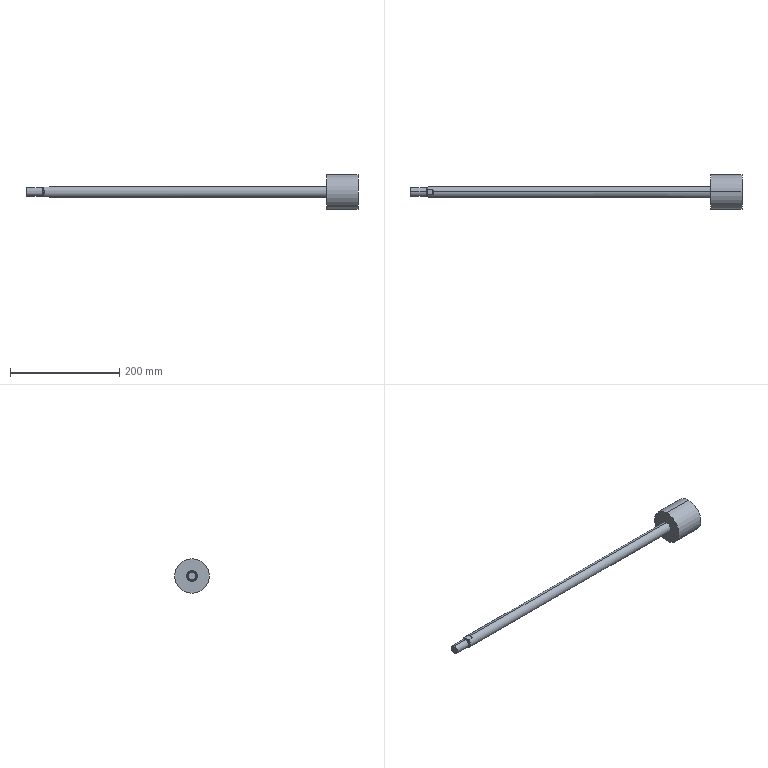Part | SolidWorks | features BaseBody 1 | 1 solid | 21 faces | box 608 x 63 x 63 mm | volume 346803 mm3 | plane 9 | cylinder 8 | cone 4 | commonest cylinder face diameters 14 x2 16 x2 20 x2 63 x2
STEP:
#1=CARTESIAN_POINT('',(482.,0.,10.));
#2=VERTEX_POINT('',#1);
#3=CARTESIAN_POINT('',(482.,0.,-10.));
#4=VERTEX_POINT('',#3);
#5=CARTESIAN_POINT('',(482.,0.,0.));
#6=DIRECTION('',(-1.,0.,0.));
#7=DIRECTION('',(0.,0.,1.));
#8=AXIS2_PLACEMENT_3D('',#5,#6,#7);
#9=CIRCLE('',#8,10.);
#10=EDGE_CURVE('',#2,#4,#9,.T.);
#11=ORIENTED_EDGE('',*,*,#10,.T.);
#12=CARTESIAN_POINT('',(-25.5,0.,-10.));
#13=VERTEX_POINT('',#12);
#14=CARTESIAN_POINT('',(539.,0.,-10.));
#15=DIRECTION('',(-1.,0.,0.));
#16=VECTOR('',#15,1000.);
#17=LINE('',#14,#16);
#18=EDGE_CURVE('',#4,#13,#17,.T.);
#19=ORIENTED_EDGE('',*,*,#18,.T.);
#20=CARTESIAN_POINT('',(-27.,5.268,-8.5));
#21=VERTEX_POINT('',#20);
#22=CARTESIAN_POINT('',(-25.5,0.,-10.));
#23=CARTESIAN_POINT('',(-25.5,1.873,-10.));
#24=CARTESIAN_POINT('',(-26.013,3.675,-9.487));
#25=CARTESIAN_POINT('',(-27.,5.268,-8.5));
#26=(BOUNDED_CURVE()B_SPLINE_CURVE(3,(#22,#23,#24,#25),.UNSPECIFIED.,.F.,.F.)B_SPLINE_CURVE_WITH_KNOTS((4,4),(3.142,3.696),.UNSPECIFIED.)CURVE()GEOMETRIC_REPRESENTATION_ITEM()RATIONAL_B_SPLINE_CURVE((1.,0.9745,0.9745,1.))REPRESENTATION_ITEM(''));
#27=EDGE_CURVE('',#13,#21,#26,.T.);
#28=ORIENTED_EDGE('',*,*,#27,.T.);
#29=CARTESIAN_POINT('',(-36.,5.268,-8.5));
#30=VERTEX_POINT('',#29);
#31=CARTESIAN_POINT('',(539.,5.268,-8.5));
#32=DIRECTION('',(-1.,0.,0.));
#33=VECTOR('',#32,1000.);
#34=LINE('',#31,#33);
#35=EDGE_CURVE('',#21,#30,#34,.T.);
#36=ORIENTED_EDGE('',*,*,#35,.T.);
#37=CARTESIAN_POINT('',(-36.,5.268,8.5));
#38=VERTEX_POINT('',#37);
#39=CARTESIAN_POINT('',(-36.,0.,0.));
#40=DIRECTION('',(1.,0.,0.));
#41=DIRECTION('',(0.,0.,1.));
#42=AXIS2_PLACEMENT_3D('',#39,#40,#41);
#43=CIRCLE('',#42,10.);
#44=EDGE_CURVE('',#30,#38,#43,.T.);
#45=ORIENTED_EDGE('',*,*,#44,.T.);
#46=CARTESIAN_POINT('',(-27.,5.268,8.5));
#47=VERTEX_POINT('',#46);
#48=CARTESIAN_POINT('',(539.,5.268,8.5));
#49=DIRECTION('',(1.,0.,0.));
#50=VECTOR('',#49,1000.);
#51=LINE('',#48,#50);
#52=EDGE_CURVE('',#38,#47,#51,.T.);
#53=ORIENTED_EDGE('',*,*,#52,.T.);
#54=CARTESIAN_POINT('',(-25.5,0.,10.));
#55=VERTEX_POINT('',#54);
#56=CARTESIAN_POINT('',(-27.,5.268,8.5));
#57=CARTESIAN_POINT('',(-26.013,3.675,9.487));
#58=CARTESIAN_POINT('',(-25.5,1.873,10.));
#59=CARTESIAN_POINT('',(-25.5,0.,10.));
#60=(BOUNDED_CURVE()B_SPLINE_CURVE(3,(#56,#57,#58,#59),.UNSPECIFIED.,.F.,.F.)B_SPLINE_CURVE_WITH_KNOTS((4,4),(2.587,3.142),.UNSPECIFIED.)CURVE()GEOMETRIC_REPRESENTATION_ITEM()RATIONAL_B_SPLINE_CURVE((1.,0.9745,0.9745,1.))REPRESENTATION_ITEM(''));
#61=EDGE_CURVE('',#47,#55,#60,.T.);
#62=ORIENTED_EDGE('',*,*,#61,.T.);
#63=CARTESIAN_POINT('',(539.,0.,10.));
#64=DIRECTION('',(-1.,0.,0.));
#65=VECTOR('',#64,1000.);
#66=LINE('',#63,#65);
#67=EDGE_CURVE('',#2,#55,#66,.T.);
#68=ORIENTED_EDGE('',*,*,#67,.F.);
#69=EDGE_LOOP('',(#11,#19,#28,#36,#45,#53,#62,#68));
#70=FACE_OUTER_BOUND('',#69,.T.);
#71=CARTESIAN_POINT('',(539.,0.,0.));
#72=DIRECTION('',(-1.,0.,0.));
#73=DIRECTION('',(0.,0.,1.));
#74=AXIS2_PLACEMENT_3D('',#71,#72,#73);
#75=CYLINDRICAL_SURFACE('',#74,10.);
#76=ADVANCED_FACE('',(#70),#75,.T.);
#77=CARTESIAN_POINT('',(539.,0.,31.5));
#78=VERTEX_POINT('',#77);
#79=CARTESIAN_POINT('',(539.,0.,-31.5));
#80=VERTEX_POINT('',#79);
#81=CARTESIAN_POINT('',(539.,0.,0.));
#82=DIRECTION('',(-1.,0.,0.));
#83=DIRECTION('',(0.,0.,1.));
#84=AXIS2_PLACEMENT_3D('',#81,#82,#83);
#85=CIRCLE('',#84,31.5);
#86=EDGE_CURVE('',#78,#80,#85,.T.);
#87=ORIENTED_EDGE('',*,*,#86,.T.);
#88=CARTESIAN_POINT('',(482.,0.,-31.5));
#89=VERTEX_POINT('',#88);
#90=CARTESIAN_POINT('',(539.,0.,-31.5));
#91=DIRECTION('',(-1.,0.,0.));
#92=VECTOR('',#91,1000.);
#93=LINE('',#90,#92);
#94=EDGE_CURVE('',#80,#89,#93,.T.);
#95=ORIENTED_EDGE('',*,*,#94,.T.);
#96=CARTESIAN_POINT('',(482.,0.,31.5));
#97=VERTEX_POINT('',#96);
#98=CARTESIAN_POINT('',(482.,0.,0.));
#99=DIRECTION('',(1.,0.,0.));
#100=DIRECTION('',(0.,0.,1.));
#101=AXIS2_PLACEMENT_3D('',#98,#99,#100);
#102=CIRCLE('',#101,31.5);
#103=EDGE_CURVE('',#89,#97,#102,.T.);
#104=ORIENTED_EDGE('',*,*,#103,.T.);
#105=CARTESIAN_POINT('',(539.,0.,31.5));
#106=DIRECTION('',(-1.,0.,0.));
#107=VECTOR('',#106,1000.);
#108=LINE('',#105,#107);
#109=EDGE_CURVE('',#78,#97,#108,.T.);
#110=ORIENTED_EDGE('',*,*,#109,.F.);
#111=EDGE_LOOP('',(#87,#95,#104,#110));
#112=FACE_OUTER_BOUND('',#111,.T.);
#113=CARTESIAN_POINT('',(539.,0.,0.));
#114=DIRECTION('',(-1.,0.,0.));
#115=DIRECTION('',(0.,0.,1.));
#116=AXIS2_PLACEMENT_3D('',#113,#114,#115);
#117=CYLINDRICAL_SURFACE('',#116,31.5);
#118=ADVANCED_FACE('',(#112),#117,.T.);
#119=CARTESIAN_POINT('',(-37.,0.,7.));
#120=VERTEX_POINT('',#119);
#121=CARTESIAN_POINT('',(-37.,0.,-7.));
#122=VERTEX_POINT('',#121);
#123=CARTESIAN_POINT('',(-37.,0.,0.));
#124=DIRECTION('',(-1.,0.,0.));
#125=DIRECTION('',(0.,0.,1.));
#126=AXIS2_PLACEMENT_3D('',#123,#124,#125);
#127=CIRCLE('',#126,7.);
#128=EDGE_CURVE('',#120,#122,#127,.T.);
#129=ORIENTED_EDGE('',*,*,#128,.T.);
#130=CARTESIAN_POINT('',(-39.,0.,-7.));
#131=VERTEX_POINT('',#130);
#132=CARTESIAN_POINT('',(539.,0.,-7.));
#133=DIRECTION('',(-1.,0.,0.));
#134=VECTOR('',#133,1000.);
#135=LINE('',#132,#134);
#136=EDGE_CURVE('',#122,#131,#135,.T.);
#137=ORIENTED_EDGE('',*,*,#136,.T.);
#138=CARTESIAN_POINT('',(-39.,0.,7.));
#139=VERTEX_POINT('',#138);
#140=CARTESIAN_POINT('',(-39.,0.,0.));
#141=DIRECTION('',(1.,0.,0.));
#142=DIRECTION('',(0.,0.,1.));
#143=AXIS2_PLACEMENT_3D('',#140,#141,#142);
#144=CIRCLE('',#143,7.);
#145=EDGE_CURVE('',#131,#139,#144,.T.);
#146=ORIENTED_EDGE('',*,*,#145,.T.);
#147=CARTESIAN_POINT('',(539.,0.,7.));
#148=DIRECTION('',(-1.,0.,0.));
#149=VECTOR('',#148,1000.);
#150=LINE('',#147,#149);
#151=EDGE_CURVE('',#120,#139,#150,.T.);
#152=ORIENTED_EDGE('',*,*,#151,.F.);
#153=EDGE_LOOP('',(#129,#137,#146,#152));
#154=FACE_OUTER_BOUND('',#153,.T.);
#155=CARTESIAN_POINT('',(539.,0.,0.));
#156=DIRECTION('',(-1.,0.,0.));
#157=DIRECTION('',(0.,0.,1.));
#158=AXIS2_PLACEMENT_3D('',#155,#156,#157);
#159=CYLINDRICAL_SURFACE('',#158,7.);
#160=ADVANCED_FACE('',(#154),#159,.T.);
#161=CARTESIAN_POINT('',(-39.,0.,8.));
#162=VERTEX_POINT('',#161);
#163=CARTESIAN_POINT('',(-39.,0.,-8.));
#164=VERTEX_POINT('',#163);
#165=CARTESIAN_POINT('',(-39.,0.,0.));
#166=DIRECTION('',(-1.,0.,0.));
#167=DIRECTION('',(0.,0.,1.));
#168=AXIS2_PLACEMENT_3D('',#165,#166,#167);
#169=CIRCLE('',#168,8.);
#170=EDGE_CURVE('',#162,#164,#169,.T.);
#171=ORIENTED_EDGE('',*,*,#170,.T.);
#172=CARTESIAN_POINT('',(-68.08,0.,-8.));
#173=VERTEX_POINT('',#172);
#174=CARTESIAN_POINT('',(539.,0.,-8.));
#175=DIRECTION('',(-1.,0.,0.));
#176=VECTOR('',#175,1000.);
#177=LINE('',#174,#176);
#178=EDGE_CURVE('',#164,#173,#177,.T.);
#179=ORIENTED_EDGE('',*,*,#178,.T.);
#180=CARTESIAN_POINT('',(-68.08,0.,8.));
#181=VERTEX_POINT('',#180);
#182=CARTESIAN_POINT('',(-68.08,0.,0.));
#183=DIRECTION('',(1.,0.,0.));
#184=DIRECTION('',(0.,0.,1.));
#185=AXIS2_PLACEMENT_3D('',#182,#183,#184);
#186=CIRCLE('',#185,8.);
#187=EDGE_CURVE('',#173,#181,#186,.T.);
#188=ORIENTED_EDGE('',*,*,#187,.T.);
#189=CARTESIAN_POINT('',(539.,0.,8.));
#190=DIRECTION('',(-1.,0.,0.));
#191=VECTOR('',#190,1000.);
#192=LINE('',#189,#191);
#193=EDGE_CURVE('',#162,#181,#192,.T.);
#194=ORIENTED_EDGE('',*,*,#193,.F.);
#195=EDGE_LOOP('',(#171,#179,#188,#194));
#196=FACE_OUTER_BOUND('',#195,.T.);
#197=CARTESIAN_POINT('',(539.,0.,0.));
#198=DIRECTION('',(-1.,0.,0.));
#199=DIRECTION('',(0.,0.,1.));
#200=AXIS2_PLACEMENT_3D('',#197,#198,#199);
#201=CYLINDRICAL_SURFACE('',#200,8.);
#202=ADVANCED_FACE('',(#196),#201,.T.);
#203=CARTESIAN_POINT('',(-69.,0.,-7.08));
#204=VERTEX_POINT('',#203);
#205=CARTESIAN_POINT('',(-69.,0.,7.08));
#206=VERTEX_POINT('',#205);
#207=CARTESIAN_POINT('',(-69.,0.,0.));
#208=DIRECTION('',(1.,0.,0.));
#209=DIRECTION('',(0.,0.,-1.));
#210=AXIS2_PLACEMENT_3D('',#207,#208,#209);
#211=CIRCLE('',#210,7.08);
#212=EDGE_CURVE('',#204,#206,#211,.T.);
#213=ORIENTED_EDGE('',*,*,#212,.T.);
#214=CARTESIAN_POINT('',(-68.08,0.,8.));
#215=DIRECTION('',(0.7071,0.,0.7071));
#216=VECTOR('',#215,1000.);
#217=LINE('',#214,#216);
#218=EDGE_CURVE('',#206,#181,#217,.T.);
#219=ORIENTED_EDGE('',*,*,#218,.T.);
#220=ORIENTED_EDGE('',*,*,#187,.F.);
#221=CARTESIAN_POINT('',(-68.08,0.,-8.));
#222=DIRECTION('',(0.7071,0.,-0.7071));
#223=VECTOR('',#222,1000.);
#224=LINE('',#221,#223);
#225=EDGE_CURVE('',#204,#173,#224,.T.);
#226=ORIENTED_EDGE('',*,*,#225,.F.);
#227=EDGE_LOOP('',(#213,#219,#220,#226));
#228=FACE_OUTER_BOUND('',#227,.T.);
#229=CARTESIAN_POINT('',(-68.08,0.,0.));
#230=DIRECTION('',(1.,0.,0.));
#231=DIRECTION('',(0.,0.,-1.));
#232=AXIS2_PLACEMENT_3D('',#229,#230,#231);
#233=CONICAL_SURFACE('',#232,8.,0.7854);
#234=ADVANCED_FACE('',(#228),#233,.T.);
#235=ORIENTED_EDGE('',*,*,#18,.F.);
#236=CARTESIAN_POINT('',(482.,0.,0.));
#237=DIRECTION('',(-1.,0.,0.));
#238=DIRECTION('',(0.,0.,1.));
#239=AXIS2_PLACEMENT_3D('',#236,#237,#238);
#240=CIRCLE('',#239,10.);
#241=EDGE_CURVE('',#4,#2,#240,.T.);
#242=ORIENTED_EDGE('',*,*,#241,.T.);
#243=ORIENTED_EDGE('',*,*,#67,.T.);
#244=CARTESIAN_POINT('',(-27.,-5.268,8.5));
#245=VERTEX_POINT('',#244);
#246=CARTESIAN_POINT('',(-25.5,0.,10.));
#247=CARTESIAN_POINT('',(-25.5,-1.873,10.));
#248=CARTESIAN_POINT('',(-26.013,-3.675,9.487));
#249=CARTESIAN_POINT('',(-27.,-5.268,8.5));
#250=(BOUNDED_CURVE()B_SPLINE_CURVE(3,(#246,#247,#248,#249),.UNSPECIFIED.,.F.,.F.)B_SPLINE_CURVE_WITH_KNOTS((4,4),(3.142,3.696),.UNSPECIFIED.)CURVE()GEOMETRIC_REPRESENTATION_ITEM()RATIONAL_B_SPLINE_CURVE((1.,0.9745,0.9745,1.))REPRESENTATION_ITEM(''));
#251=EDGE_CURVE('',#55,#245,#250,.T.);
#252=ORIENTED_EDGE('',*,*,#251,.T.);
#253=CARTESIAN_POINT('',(-36.,-5.268,8.5));
#254=VERTEX_POINT('',#253);
#255=CARTESIAN_POINT('',(539.,-5.268,8.5));
#256=DIRECTION('',(-1.,0.,0.));
#257=VECTOR('',#256,1000.);
#258=LINE('',#255,#257);
#259=EDGE_CURVE('',#245,#254,#258,.T.);
#260=ORIENTED_EDGE('',*,*,#259,.T.);
#261=CARTESIAN_POINT('',(-36.,-5.268,-8.5));
#262=VERTEX_POINT('',#261);
#263=CARTESIAN_POINT('',(-36.,0.,0.));
#264=DIRECTION('',(1.,0.,0.));
#265=DIRECTION('',(0.,0.,1.));
#266=AXIS2_PLACEMENT_3D('',#263,#264,#265);
#267=CIRCLE('',#266,10.);
#268=EDGE_CURVE('',#254,#262,#267,.T.);
#269=ORIENTED_EDGE('',*,*,#268,.T.);
#270=CARTESIAN_POINT('',(-27.,-5.268,-8.5));
#271=VERTEX_POINT('',#270);
#272=CARTESIAN_POINT('',(539.,-5.268,-8.5));
#273=DIRECTION('',(1.,0.,0.));
#274=VECTOR('',#273,1000.);
#275=LINE('',#272,#274);
#276=EDGE_CURVE('',#262,#271,#275,.T.);
#277=ORIENTED_EDGE('',*,*,#276,.T.);
#278=CARTESIAN_POINT('',(-27.,-5.268,-8.5));
#279=CARTESIAN_POINT('',(-26.013,-3.675,-9.487));
#280=CARTESIAN_POINT('',(-25.5,-1.873,-10.));
#281=CARTESIAN_POINT('',(-25.5,0.,-10.));
#282=(BOUNDED_CURVE()B_SPLINE_CURVE(3,(#278,#279,#280,#281),.UNSPECIFIED.,.F.,.F.)B_SPLINE_CURVE_WITH_KNOTS((4,4),(2.587,3.142),.UNSPECIFIED.)CURVE()GEOMETRIC_REPRESENTATION_ITEM()RATIONAL_B_SPLINE_CURVE((1.,0.9745,0.9745,1.))REPRESENTATION_ITEM(''));
#283=EDGE_CURVE('',#271,#13,#282,.T.);
#284=ORIENTED_EDGE('',*,*,#283,.T.);
#285=EDGE_LOOP('',(#235,#242,#243,#252,#260,#269,#277,#284));
#286=FACE_OUTER_BOUND('',#285,.T.);
#287=CARTESIAN_POINT('',(539.,0.,0.));
#288=DIRECTION('',(-1.,0.,0.));
#289=DIRECTION('',(0.,0.,1.));
#290=AXIS2_PLACEMENT_3D('',#287,#288,#289);
#291=CYLINDRICAL_SURFACE('',#290,10.);
#292=ADVANCED_FACE('',(#286),#291,.T.);
#293=ORIENTED_EDGE('',*,*,#61,.F.);
#294=CARTESIAN_POINT('',(-27.,20.,8.5));
#295=DIRECTION('',(0.,-1.,0.));
#296=VECTOR('',#295,1000.);
#297=LINE('',#294,#296);
#298=EDGE_CURVE('',#47,#245,#297,.T.);
#299=ORIENTED_EDGE('',*,*,#298,.T.);
#300=ORIENTED_EDGE('',*,*,#251,.F.);
#301=EDGE_LOOP('',(#293,#299,#300));
#302=FACE_OUTER_BOUND('',#301,.T.);
#303=CARTESIAN_POINT('',(-11.393,20.,24.107));
#304=DIRECTION('',(-0.7071,0.,0.7071));
#305=DIRECTION('',(0.7071,0.,0.7071));
#306=AXIS2_PLACEMENT_3D('',#303,#304,#305);
#307=PLANE('',#306);
#308=ADVANCED_FACE('',(#302),#307,.T.);
#309=CARTESIAN_POINT('',(-37.,2.958,8.5));
#310=VERTEX_POINT('',#309);
#311=CARTESIAN_POINT('',(-36.,5.268,8.5));
#312=CARTESIAN_POINT('',(-36.392,4.523,8.5));
#313=CARTESIAN_POINT('',(-36.737,3.758,8.5));
#314=CARTESIAN_POINT('',(-37.,2.958,8.5));
#315=B_SPLINE_CURVE_WITH_KNOTS('',3,(#311,#312,#313,#314),.UNSPECIFIED.,.F.,.F.,(4,4),(0.,0.002517),.UNSPECIFIED.);
#316=EDGE_CURVE('',#38,#310,#315,.T.);
#317=ORIENTED_EDGE('',*,*,#316,.T.);
#318=CARTESIAN_POINT('',(-37.,-2.958,8.5));
#319=VERTEX_POINT('',#318);
#320=CARTESIAN_POINT('',(-37.,20.,8.5));
#321=DIRECTION('',(0.,-1.,0.));
#322=VECTOR('',#321,1000.);
#323=LINE('',#320,#322);
#324=EDGE_CURVE('',#310,#319,#323,.T.);
#325=ORIENTED_EDGE('',*,*,#324,.T.);
#326=CARTESIAN_POINT('',(-37.,-2.958,8.5));
#327=CARTESIAN_POINT('',(-36.737,-3.758,8.5));
#328=CARTESIAN_POINT('',(-36.392,-4.523,8.5));
#329=CARTESIAN_POINT('',(-36.,-5.268,8.5));
#330=B_SPLINE_CURVE_WITH_KNOTS('',3,(#326,#327,#328,#329),.UNSPECIFIED.,.F.,.F.,(4,4),(0.,0.002517),.UNSPECIFIED.);
#331=EDGE_CURVE('',#319,#254,#330,.T.);
#332=ORIENTED_EDGE('',*,*,#331,.T.);
#333=ORIENTED_EDGE('',*,*,#259,.F.);
#334=ORIENTED_EDGE('',*,*,#298,.F.);
#335=ORIENTED_EDGE('',*,*,#52,.F.);
#336=EDGE_LOOP('',(#317,#325,#332,#333,#334,#335));
#337=FACE_OUTER_BOUND('',#336,.T.);
#338=CARTESIAN_POINT('',(-27.,20.,8.5));
#339=DIRECTION('',(0.,0.,1.));
#340=DIRECTION('',(1.,0.,0.));
#341=AXIS2_PLACEMENT_3D('',#338,#339,#340);
#342=PLANE('',#341);
#343=ADVANCED_FACE('',(#337),#342,.T.);
#344=ORIENTED_EDGE('',*,*,#316,.F.);
#345=ORIENTED_EDGE('',*,*,#44,.F.);
#346=CARTESIAN_POINT('',(-37.,2.958,-8.5));
#347=VERTEX_POINT('',#346);
#348=CARTESIAN_POINT('',(-36.,5.268,-8.5));
#349=CARTESIAN_POINT('',(-36.392,4.523,-8.5));
#350=CARTESIAN_POINT('',(-36.737,3.758,-8.5));
#351=CARTESIAN_POINT('',(-37.,2.958,-8.5));
#352=B_SPLINE_CURVE_WITH_KNOTS('',3,(#348,#349,#350,#351),.UNSPECIFIED.,.F.,.F.,(4,4),(0.,0.002517),.UNSPECIFIED.);
#353=EDGE_CURVE('',#30,#347,#352,.T.);
#354=ORIENTED_EDGE('',*,*,#353,.T.);
#355=CARTESIAN_POINT('',(-37.,0.,0.));
#356=DIRECTION('',(1.,0.,0.));
#357=DIRECTION('',(0.,0.,-1.));
#358=AXIS2_PLACEMENT_3D('',#355,#356,#357);
#359=CIRCLE('',#358,9.);
#360=EDGE_CURVE('',#347,#310,#359,.T.);
#361=ORIENTED_EDGE('',*,*,#360,.T.);
#362=EDGE_LOOP('',(#344,#345,#354,#361));
#363=FACE_OUTER_BOUND('',#362,.T.);
#364=CARTESIAN_POINT('',(-36.,0.,0.));
#365=DIRECTION('',(1.,0.,0.));
#366=DIRECTION('',(0.,0.,-1.));
#367=AXIS2_PLACEMENT_3D('',#364,#365,#366);
#368=CONICAL_SURFACE('',#367,10.,0.7854);
#369=ADVANCED_FACE('',(#363),#368,.T.);
#370=CARTESIAN_POINT('',(-37.,-2.958,-8.5));
#371=VERTEX_POINT('',#370);
#372=CARTESIAN_POINT('',(-36.,-5.268,-8.5));
#373=CARTESIAN_POINT('',(-36.392,-4.523,-8.5));
#374=CARTESIAN_POINT('',(-36.737,-3.758,-8.5));
#375=CARTESIAN_POINT('',(-37.,-2.958,-8.5));
#376=B_SPLINE_CURVE_WITH_KNOTS('',3,(#372,#373,#374,#375),.UNSPECIFIED.,.F.,.F.,(4,4),(0.,0.002517),.UNSPECIFIED.);
#377=EDGE_CURVE('',#262,#371,#376,.T.);
#378=ORIENTED_EDGE('',*,*,#377,.T.);
#379=CARTESIAN_POINT('',(-37.,20.,-8.5));
#380=DIRECTION('',(0.,1.,0.));
#381=VECTOR('',#380,1000.);
#382=LINE('',#379,#381);
#383=EDGE_CURVE('',#371,#347,#382,.T.);
#384=ORIENTED_EDGE('',*,*,#383,.T.);
#385=ORIENTED_EDGE('',*,*,#353,.F.);
#386=ORIENTED_EDGE('',*,*,#35,.F.);
#387=CARTESIAN_POINT('',(-27.,20.,-8.5));
#388=DIRECTION('',(0.,-1.,0.));
#389=VECTOR('',#388,1000.);
#390=LINE('',#387,#389);
#391=EDGE_CURVE('',#21,#271,#390,.T.);
#392=ORIENTED_EDGE('',*,*,#391,.T.);
#393=ORIENTED_EDGE('',*,*,#276,.F.);
#394=EDGE_LOOP('',(#378,#384,#385,#386,#392,#393));
#395=FACE_OUTER_BOUND('',#394,.T.);
#396=CARTESIAN_POINT('',(-37.,20.,-8.5));
#397=DIRECTION('',(0.,0.,-1.));
#398=DIRECTION('',(-1.,0.,0.));
#399=AXIS2_PLACEMENT_3D('',#396,#397,#398);
#400=PLANE('',#399);
#401=ADVANCED_FACE('',(#395),#400,.T.);
#402=ORIENTED_EDGE('',*,*,#283,.F.);
#403=ORIENTED_EDGE('',*,*,#391,.F.);
#404=ORIENTED_EDGE('',*,*,#27,.F.);
#405=EDGE_LOOP('',(#402,#403,#404));
#406=FACE_OUTER_BOUND('',#405,.T.);
#407=CARTESIAN_POINT('',(-27.,20.,-8.5));
#408=DIRECTION('',(-0.7071,0.,-0.7071));
#409=DIRECTION('',(-0.7071,0.,0.7071));
#410=AXIS2_PLACEMENT_3D('',#407,#408,#409);
#411=PLANE('',#410);
#412=ADVANCED_FACE('',(#406),#411,.T.);
#413=ORIENTED_EDGE('',*,*,#377,.F.);
#414=ORIENTED_EDGE('',*,*,#268,.F.);
#415=ORIENTED_EDGE('',*,*,#331,.F.);
#416=CARTESIAN_POINT('',(-37.,0.,0.));
#417=DIRECTION('',(1.,0.,0.));
#418=DIRECTION('',(0.,0.,-1.));
#419=AXIS2_PLACEMENT_3D('',#416,#417,#418);
#420=CIRCLE('',#419,9.);
#421=EDGE_CURVE('',#319,#371,#420,.T.);
#422=ORIENTED_EDGE('',*,*,#421,.T.);
#423=EDGE_LOOP('',(#413,#414,#415,#422));
#424=FACE_OUTER_BOUND('',#423,.T.);
#425=CARTESIAN_POINT('',(-36.,0.,0.));
#426=DIRECTION('',(1.,0.,0.));
#427=DIRECTION('',(0.,0.,-1.));
#428=AXIS2_PLACEMENT_3D('',#425,#426,#427);
#429=CONICAL_SURFACE('',#428,10.,0.7854);
#430=ADVANCED_FACE('',(#424),#429,.T.);
#431=ORIENTED_EDGE('',*,*,#10,.F.);
#432=ORIENTED_EDGE('',*,*,#241,.F.);
#433=EDGE_LOOP('',(#431,#432));
#434=FACE_BOUND('',#433,.T.);
#435=CARTESIAN_POINT('',(482.,0.,0.));
#436=DIRECTION('',(1.,0.,0.));
#437=DIRECTION('',(0.,0.,1.));
#438=AXIS2_PLACEMENT_3D('',#435,#436,#437);
#439=CIRCLE('',#438,31.5);
#440=EDGE_CURVE('',#97,#89,#439,.T.);
#441=ORIENTED_EDGE('',*,*,#440,.F.);
#442=ORIENTED_EDGE('',*,*,#103,.F.);
#443=EDGE_LOOP('',(#441,#442));
#444=FACE_OUTER_BOUND('',#443,.T.);
#445=CARTESIAN_POINT('',(482.,10.,0.));
#446=DIRECTION('',(1.,0.,0.));
#447=DIRECTION('',(0.,0.,-1.));
#448=AXIS2_PLACEMENT_3D('',#445,#446,#447);
#449=PLANE('',#448);
#450=ADVANCED_FACE('',(#434,#444),#449,.F.);
#451=ORIENTED_EDGE('',*,*,#128,.F.);
#452=CARTESIAN_POINT('',(-37.,0.,0.));
#453=DIRECTION('',(-1.,0.,0.));
#454=DIRECTION('',(0.,0.,1.));
#455=AXIS2_PLACEMENT_3D('',#452,#453,#454);
#456=CIRCLE('',#455,7.);
#457=EDGE_CURVE('',#122,#120,#456,.T.);
#458=ORIENTED_EDGE('',*,*,#457,.F.);
#459=EDGE_LOOP('',(#451,#458));
#460=FACE_BOUND('',#459,.T.);
#461=ORIENTED_EDGE('',*,*,#383,.F.);
#462=ORIENTED_EDGE('',*,*,#421,.F.);
#463=ORIENTED_EDGE('',*,*,#324,.F.);
#464=ORIENTED_EDGE('',*,*,#360,.F.);
#465=EDGE_LOOP('',(#461,#462,#463,#464));
#466=FACE_OUTER_BOUND('',#465,.T.);
#467=CARTESIAN_POINT('',(-37.,7.,0.));
#468=DIRECTION('',(1.,0.,0.));
#469=DIRECTION('',(0.,0.,-1.));
#470=AXIS2_PLACEMENT_3D('',#467,#468,#469);
#471=PLANE('',#470);
#472=ADVANCED_FACE('',(#460,#466),#471,.F.);
#473=ORIENTED_EDGE('',*,*,#94,.F.);
#474=CARTESIAN_POINT('',(539.,0.,0.));
#475=DIRECTION('',(-1.,0.,0.));
#476=DIRECTION('',(0.,0.,1.));
#477=AXIS2_PLACEMENT_3D('',#474,#475,#476);
#478=CIRCLE('',#477,31.5);
#479=EDGE_CURVE('',#80,#78,#478,.T.);
#480=ORIENTED_EDGE('',*,*,#479,.T.);
#481=ORIENTED_EDGE('',*,*,#109,.T.);
#482=ORIENTED_EDGE('',*,*,#440,.T.);
#483=EDGE_LOOP('',(#473,#480,#481,#482));
#484=FACE_OUTER_BOUND('',#483,.T.);
#485=CARTESIAN_POINT('',(539.,0.,0.));
#486=DIRECTION('',(-1.,0.,0.));
#487=DIRECTION('',(0.,0.,1.));
#488=AXIS2_PLACEMENT_3D('',#485,#486,#487);
#489=CYLINDRICAL_SURFACE('',#488,31.5);
#490=ADVANCED_FACE('',(#484),#489,.T.);
#491=ORIENTED_EDGE('',*,*,#136,.F.);
#492=ORIENTED_EDGE('',*,*,#457,.T.);
#493=ORIENTED_EDGE('',*,*,#151,.T.);
#494=CARTESIAN_POINT('',(-39.,0.,0.));
#495=DIRECTION('',(1.,0.,0.));
#496=DIRECTION('',(0.,0.,1.));
#497=AXIS2_PLACEMENT_3D('',#494,#495,#496);
#498=CIRCLE('',#497,7.);
#499=EDGE_CURVE('',#139,#131,#498,.T.);
#500=ORIENTED_EDGE('',*,*,#499,.T.);
#501=EDGE_LOOP('',(#491,#492,#493,#500));
#502=FACE_OUTER_BOUND('',#501,.T.);
#503=CARTESIAN_POINT('',(539.,0.,0.));
#504=DIRECTION('',(-1.,0.,0.));
#505=DIRECTION('',(0.,0.,1.));
#506=AXIS2_PLACEMENT_3D('',#503,#504,#505);
#507=CYLINDRICAL_SURFACE('',#506,7.);
#508=ADVANCED_FACE('',(#502),#507,.T.);
#509=ORIENTED_EDGE('',*,*,#86,.F.);
#510=ORIENTED_EDGE('',*,*,#479,.F.);
#511=EDGE_LOOP('',(#509,#510));
#512=FACE_OUTER_BOUND('',#511,.T.);
#513=CARTESIAN_POINT('',(539.,31.5,0.));
#514=DIRECTION('',(-1.,0.,0.));
#515=DIRECTION('',(0.,0.,1.));
#516=AXIS2_PLACEMENT_3D('',#513,#514,#515);
#517=PLANE('',#516);
#518=ADVANCED_FACE('',(#512),#517,.F.);
#519=ORIENTED_EDGE('',*,*,#170,.F.);
#520=CARTESIAN_POINT('',(-39.,0.,0.));
#521=DIRECTION('',(-1.,0.,0.));
#522=DIRECTION('',(0.,0.,1.));
#523=AXIS2_PLACEMENT_3D('',#520,#521,#522);
#524=CIRCLE('',#523,8.);
#525=EDGE_CURVE('',#164,#162,#524,.T.);
#526=ORIENTED_EDGE('',*,*,#525,.F.);
#527=EDGE_LOOP('',(#519,#526));
#528=FACE_OUTER_BOUND('',#527,.T.);
#529=ORIENTED_EDGE('',*,*,#499,.F.);
#530=ORIENTED_EDGE('',*,*,#145,.F.);
#531=EDGE_LOOP('',(#529,#530));
#532=FACE_BOUND('',#531,.T.);
#533=CARTESIAN_POINT('',(-39.,8.,0.));
#534=DIRECTION('',(-1.,0.,0.));
#535=DIRECTION('',(0.,0.,1.));
#536=AXIS2_PLACEMENT_3D('',#533,#534,#535);
#537=PLANE('',#536);
#538=ADVANCED_FACE('',(#528,#532),#537,.F.);
#539=ORIENTED_EDGE('',*,*,#178,.F.);
#540=ORIENTED_EDGE('',*,*,#525,.T.);
#541=ORIENTED_EDGE('',*,*,#193,.T.);
#542=CARTESIAN_POINT('',(-68.08,0.,0.));
#543=DIRECTION('',(1.,0.,0.));
#544=DIRECTION('',(0.,0.,1.));
#545=AXIS2_PLACEMENT_3D('',#542,#543,#544);
#546=CIRCLE('',#545,8.);
#547=EDGE_CURVE('',#181,#173,#546,.T.);
#548=ORIENTED_EDGE('',*,*,#547,.T.);
#549=EDGE_LOOP('',(#539,#540,#541,#548));
#550=FACE_OUTER_BOUND('',#549,.T.);
#551=CARTESIAN_POINT('',(539.,0.,0.));
#552=DIRECTION('',(-1.,0.,0.));
#553=DIRECTION('',(0.,0.,1.));
#554=AXIS2_PLACEMENT_3D('',#551,#552,#553);
#555=CYLINDRICAL_SURFACE('',#554,8.);
#556=ADVANCED_FACE('',(#550),#555,.T.);
#557=ORIENTED_EDGE('',*,*,#218,.F.);
#558=CARTESIAN_POINT('',(-69.,0.,0.));
#559=DIRECTION('',(1.,0.,0.));
#560=DIRECTION('',(0.,0.,-1.));
#561=AXIS2_PLACEMENT_3D('',#558,#559,#560);
#562=CIRCLE('',#561,7.08);
#563=EDGE_CURVE('',#206,#204,#562,.T.);
#564=ORIENTED_EDGE('',*,*,#563,.T.);
#565=ORIENTED_EDGE('',*,*,#225,.T.);
#566=ORIENTED_EDGE('',*,*,#547,.F.);
#567=EDGE_LOOP('',(#557,#564,#565,#566));
#568=FACE_OUTER_BOUND('',#567,.T.);
#569=CARTESIAN_POINT('',(-68.08,0.,0.));
#570=DIRECTION('',(1.,0.,0.));
#571=DIRECTION('',(0.,0.,-1.));
#572=AXIS2_PLACEMENT_3D('',#569,#570,#571);
#573=CONICAL_SURFACE('',#572,8.,0.7854);
#574=ADVANCED_FACE('',(#568),#573,.T.);
#575=ORIENTED_EDGE('',*,*,#212,.F.);
#576=ORIENTED_EDGE('',*,*,#563,.F.);
#577=EDGE_LOOP('',(#575,#576));
#578=FACE_OUTER_BOUND('',#577,.T.);
#579=CARTESIAN_POINT('',(-69.,0.,0.));
#580=DIRECTION('',(1.,0.,0.));
#581=DIRECTION('',(0.,0.,-1.));
#582=AXIS2_PLACEMENT_3D('',#579,#580,#581);
#583=PLANE('',#582);
#584=ADVANCED_FACE('',(#578),#583,.F.);
#585=CLOSED_SHELL('',(#76,#118,#160,#202,#234,#292,#308,#343,#369,#401,#412,#430,#450,#472,#490,#508,#518,#538,#556,#574,#584));
#586=MANIFOLD_SOLID_BREP('',#585);
#587=CARTESIAN_POINT('',(0.,0.,0.));
#588=DIRECTION('',(0.,0.,1.));
#589=DIRECTION('',(1.,0.,0.));
#590=AXIS2_PLACEMENT_3D('',#587,#588,#589);
#591=(LENGTH_UNIT()NAMED_UNIT(*)SI_UNIT(.MILLI.,.METRE.));
#592=UNCERTAINTY_MEASURE_WITH_UNIT(LENGTH_MEASURE(0.00001),#591,'','');
#593=(NAMED_UNIT(*)PLANE_ANGLE_UNIT()SI_UNIT($,.RADIAN.));
#594=(NAMED_UNIT(*)SI_UNIT($,.STERADIAN.)SOLID_ANGLE_UNIT());
#595=(GEOMETRIC_REPRESENTATION_CONTEXT(3)GLOBAL_UNCERTAINTY_ASSIGNED_CONTEXT((#592))GLOBAL_UNIT_ASSIGNED_CONTEXT((#591,#593,#594))REPRESENTATION_CONTEXT('',''));
#596=ADVANCED_BREP_SHAPE_REPRESENTATION('',(#586,#590),#595);